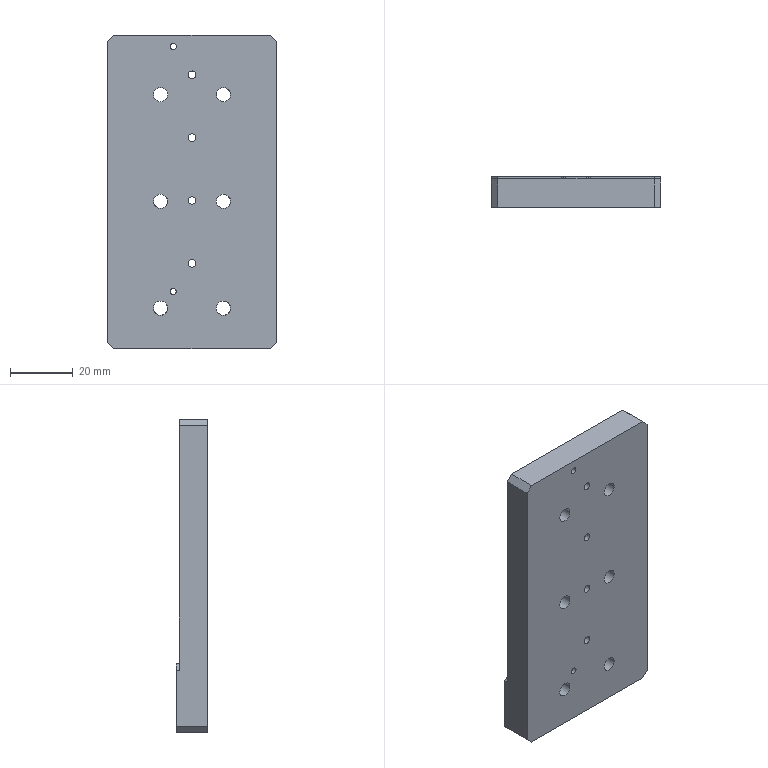Part | 1 solid | 52 faces | box 54 x 10 x 100 mm | volume 47425 mm3 | plane 26 | cylinder 26 | commonest cylinder face diameters 2 x6 4.5 x6 8 x6 2.5 x4 1 x2 3 x2
STEP:
#1=CARTESIAN_POINT('',(137.424,25.392,-106.529));
#2=VERTEX_POINT('',#1);
#3=CARTESIAN_POINT('',(116.923,25.392,-106.529));
#4=VERTEX_POINT('',#3);
#5=CARTESIAN_POINT('',(114.923,25.392,-106.529));
#6=DIRECTION('',(-1.,-0.000000698,0.));
#7=VECTOR('',#6,1000.);
#8=LINE('',#5,#7);
#9=EDGE_CURVE('',#2,#4,#8,.T.);
#10=ORIENTED_EDGE('',*,*,#9,.F.);
#11=CARTESIAN_POINT('',(137.424,26.392,-106.529));
#12=VERTEX_POINT('',#11);
#13=CARTESIAN_POINT('',(137.424,25.892,-106.529));
#14=DIRECTION('',(-0.000000698,1.,0.));
#15=VECTOR('',#14,1000.);
#16=LINE('',#13,#15);
#17=EDGE_CURVE('',#2,#12,#16,.T.);
#18=ORIENTED_EDGE('',*,*,#17,.T.);
#19=CARTESIAN_POINT('',(116.923,26.392,-106.529));
#20=VERTEX_POINT('',#19);
#21=CARTESIAN_POINT('',(114.923,26.392,-106.529));
#22=DIRECTION('',(-1.,-0.000000698,0.));
#23=VECTOR('',#22,1000.);
#24=LINE('',#21,#23);
#25=EDGE_CURVE('',#12,#20,#24,.T.);
#26=ORIENTED_EDGE('',*,*,#25,.T.);
#27=CARTESIAN_POINT('',(116.923,25.392,-106.529));
#28=DIRECTION('',(0.000000698,-1.,0.));
#29=VECTOR('',#28,1000.);
#30=LINE('',#27,#29);
#31=EDGE_CURVE('',#20,#4,#30,.T.);
#32=ORIENTED_EDGE('',*,*,#31,.T.);
#33=EDGE_LOOP('',(#10,#18,#26,#32));
#34=FACE_BOUND('',#33,.T.);
#35=CARTESIAN_POINT('',(114.923,25.392,-106.529));
#36=DIRECTION('',(0.,0.,-1.));
#37=DIRECTION('',(0.,-1.,0.));
#38=AXIS2_PLACEMENT_3D('',#35,#36,#37);
#39=PLANE('',#38);
#40=ADVANCED_FACE('',(#34),#39,.F.);
#41=CARTESIAN_POINT('',(135.923,26.392,-111.729));
#42=VERTEX_POINT('',#41);
#43=CARTESIAN_POINT('',(135.923,26.392,-110.229));
#44=DIRECTION('',(0.000000698,-1.,0.));
#45=DIRECTION('',(-0.000000349,0.,-1.));
#46=AXIS2_PLACEMENT_3D('',#43,#44,#45);
#47=CIRCLE('',#46,1.5);
#48=EDGE_CURVE('',#42,#42,#47,.T.);
#49=ORIENTED_EDGE('',*,*,#48,.T.);
#50=EDGE_LOOP('',(#49));
#51=FACE_BOUND('',#50,.T.);
#52=CARTESIAN_POINT('',(151.923,26.392,-111.529));
#53=VERTEX_POINT('',#52);
#54=CARTESIAN_POINT('',(151.923,26.392,-115.529));
#55=DIRECTION('',(-0.000000698,1.,0.));
#56=DIRECTION('',(0.,0.,1.));
#57=AXIS2_PLACEMENT_3D('',#54,#55,#56);
#58=CIRCLE('',#57,4.);
#59=EDGE_CURVE('',#53,#53,#58,.T.);
#60=ORIENTED_EDGE('',*,*,#59,.F.);
#61=EDGE_LOOP('',(#60));
#62=FACE_BOUND('',#61,.T.);
#63=CARTESIAN_POINT('',(131.923,26.392,-111.529));
#64=VERTEX_POINT('',#63);
#65=CARTESIAN_POINT('',(131.923,26.392,-115.529));
#66=DIRECTION('',(-0.000000698,1.,0.));
#67=DIRECTION('',(0.,0.,1.));
#68=AXIS2_PLACEMENT_3D('',#65,#66,#67);
#69=CIRCLE('',#68,4.);
#70=EDGE_CURVE('',#64,#64,#69,.T.);
#71=ORIENTED_EDGE('',*,*,#70,.F.);
#72=EDGE_LOOP('',(#71));
#73=FACE_BOUND('',#72,.T.);
#74=CARTESIAN_POINT('',(146.051,26.392,-109.062));
#75=VERTEX_POINT('',#74);
#76=CARTESIAN_POINT('',(146.757,26.392,-108.356));
#77=VERTEX_POINT('',#76);
#78=CARTESIAN_POINT('',(146.424,26.392,-108.729));
#79=DIRECTION('',(0.000000698,-1.,0.));
#80=DIRECTION('',(-0.000000349,0.,-1.));
#81=AXIS2_PLACEMENT_3D('',#78,#79,#80);
#82=CIRCLE('',#81,0.5);
#83=EDGE_CURVE('',#75,#77,#82,.T.);
#84=ORIENTED_EDGE('',*,*,#83,.T.);
#85=CARTESIAN_POINT('',(146.424,26.392,-107.611));
#86=VERTEX_POINT('',#85);
#87=CARTESIAN_POINT('',(147.424,26.392,-107.611));
#88=DIRECTION('',(0.000000698,-1.,0.));
#89=DIRECTION('',(1.,0.000000698,0.));
#90=AXIS2_PLACEMENT_3D('',#87,#88,#89);
#91=CIRCLE('',#90,1.);
#92=EDGE_CURVE('',#77,#86,#91,.F.);
#93=ORIENTED_EDGE('',*,*,#92,.T.);
#94=CARTESIAN_POINT('',(146.424,26.392,-106.529));
#95=VERTEX_POINT('',#94);
#96=CARTESIAN_POINT('',(146.424,26.392,-77.529));
#97=DIRECTION('',(0.,0.,-1.));
#98=VECTOR('',#97,1000.);
#99=LINE('',#96,#98);
#100=EDGE_CURVE('',#95,#86,#99,.T.);
#101=ORIENTED_EDGE('',*,*,#100,.F.);
#102=CARTESIAN_POINT('',(166.923,26.392,-106.529));
#103=VERTEX_POINT('',#102);
#104=CARTESIAN_POINT('',(114.923,26.392,-106.529));
#105=DIRECTION('',(-1.,-0.000000698,0.));
#106=VECTOR('',#105,1000.);
#107=LINE('',#104,#106);
#108=EDGE_CURVE('',#103,#95,#107,.T.);
#109=ORIENTED_EDGE('',*,*,#108,.F.);
#110=CARTESIAN_POINT('',(168.923,26.392,-108.529));
#111=VERTEX_POINT('',#110);
#112=CARTESIAN_POINT('',(166.923,26.392,-106.529));
#113=DIRECTION('',(0.7071,0.000000494,-0.7071));
#114=VECTOR('',#113,1000.);
#115=LINE('',#112,#114);
#116=EDGE_CURVE('',#103,#111,#115,.T.);
#117=ORIENTED_EDGE('',*,*,#116,.T.);
#118=CARTESIAN_POINT('',(168.923,26.392,-126.529));
#119=VERTEX_POINT('',#118);
#120=CARTESIAN_POINT('',(168.923,26.392,-128.529));
#121=DIRECTION('',(0.,0.,1.));
#122=VECTOR('',#121,1000.);
#123=LINE('',#120,#122);
#124=EDGE_CURVE('',#119,#111,#123,.T.);
#125=ORIENTED_EDGE('',*,*,#124,.F.);
#126=CARTESIAN_POINT('',(166.923,26.392,-128.529));
#127=VERTEX_POINT('',#126);
#128=CARTESIAN_POINT('',(168.923,26.392,-126.529));
#129=DIRECTION('',(-0.7071,-0.000000494,-0.7071));
#130=VECTOR('',#129,1000.);
#131=LINE('',#128,#130);
#132=EDGE_CURVE('',#119,#127,#131,.T.);
#133=ORIENTED_EDGE('',*,*,#132,.T.);
#134=CARTESIAN_POINT('',(116.923,26.392,-128.529));
#135=VERTEX_POINT('',#134);
#136=CARTESIAN_POINT('',(114.923,26.392,-128.529));
#137=DIRECTION('',(1.,0.000000698,0.));
#138=VECTOR('',#137,1000.);
#139=LINE('',#136,#138);
#140=EDGE_CURVE('',#135,#127,#139,.T.);
#141=ORIENTED_EDGE('',*,*,#140,.F.);
#142=CARTESIAN_POINT('',(114.923,26.392,-126.529));
#143=VERTEX_POINT('',#142);
#144=CARTESIAN_POINT('',(116.923,26.392,-128.529));
#145=DIRECTION('',(-0.7071,-0.000000494,0.7071));
#146=VECTOR('',#145,1000.);
#147=LINE('',#144,#146);
#148=EDGE_CURVE('',#135,#143,#147,.T.);
#149=ORIENTED_EDGE('',*,*,#148,.T.);
#150=CARTESIAN_POINT('',(114.923,26.392,-108.529));
#151=VERTEX_POINT('',#150);
#152=CARTESIAN_POINT('',(114.923,26.392,-128.529));
#153=DIRECTION('',(0.,0.,-1.));
#154=VECTOR('',#153,1000.);
#155=LINE('',#152,#154);
#156=EDGE_CURVE('',#151,#143,#155,.T.);
#157=ORIENTED_EDGE('',*,*,#156,.F.);
#158=CARTESIAN_POINT('',(114.923,26.392,-108.529));
#159=DIRECTION('',(0.7071,0.000000494,0.7071));
#160=VECTOR('',#159,1000.);
#161=LINE('',#158,#160);
#162=EDGE_CURVE('',#151,#20,#161,.T.);
#163=ORIENTED_EDGE('',*,*,#162,.T.);
#164=ORIENTED_EDGE('',*,*,#25,.F.);
#165=CARTESIAN_POINT('',(137.424,26.392,-107.611));
#166=VERTEX_POINT('',#165);
#167=CARTESIAN_POINT('',(137.424,26.392,-77.529));
#168=DIRECTION('',(0.,0.,1.));
#169=VECTOR('',#168,1000.);
#170=LINE('',#167,#169);
#171=EDGE_CURVE('',#166,#12,#170,.T.);
#172=ORIENTED_EDGE('',*,*,#171,.F.);
#173=CARTESIAN_POINT('',(137.091,26.392,-108.357));
#174=VERTEX_POINT('',#173);
#175=CARTESIAN_POINT('',(136.424,26.392,-107.611));
#176=DIRECTION('',(0.000000698,-1.,0.));
#177=DIRECTION('',(1.,0.000000698,0.));
#178=AXIS2_PLACEMENT_3D('',#175,#176,#177);
#179=CIRCLE('',#178,1.);
#180=EDGE_CURVE('',#166,#174,#179,.F.);
#181=ORIENTED_EDGE('',*,*,#180,.T.);
#182=CARTESIAN_POINT('',(137.797,26.392,-109.063));
#183=VERTEX_POINT('',#182);
#184=CARTESIAN_POINT('',(137.424,26.392,-108.729));
#185=DIRECTION('',(0.000000698,-1.,0.));
#186=DIRECTION('',(-0.000000349,0.,-1.));
#187=AXIS2_PLACEMENT_3D('',#184,#185,#186);
#188=CIRCLE('',#187,0.5);
#189=EDGE_CURVE('',#174,#183,#188,.T.);
#190=ORIENTED_EDGE('',*,*,#189,.T.);
#191=CARTESIAN_POINT('',(138.542,26.392,-108.729));
#192=VERTEX_POINT('',#191);
#193=CARTESIAN_POINT('',(138.542,26.392,-109.729));
#194=DIRECTION('',(0.000000698,-1.,0.));
#195=DIRECTION('',(1.,0.000000698,0.));
#196=AXIS2_PLACEMENT_3D('',#193,#194,#195);
#197=CIRCLE('',#196,1.);
#198=EDGE_CURVE('',#183,#192,#197,.F.);
#199=ORIENTED_EDGE('',*,*,#198,.T.);
#200=CARTESIAN_POINT('',(145.306,26.392,-108.729));
#201=VERTEX_POINT('',#200);
#202=CARTESIAN_POINT('',(141.925,26.392,-108.729));
#203=DIRECTION('',(-1.,-0.000000698,0.));
#204=VECTOR('',#203,1000.);
#205=LINE('',#202,#204);
#206=EDGE_CURVE('',#201,#192,#205,.T.);
#207=ORIENTED_EDGE('',*,*,#206,.F.);
#208=CARTESIAN_POINT('',(145.306,26.392,-109.729));
#209=DIRECTION('',(0.000000698,-1.,0.));
#210=DIRECTION('',(1.,0.000000698,0.));
#211=AXIS2_PLACEMENT_3D('',#208,#209,#210);
#212=CIRCLE('',#211,1.);
#213=EDGE_CURVE('',#201,#75,#212,.F.);
#214=ORIENTED_EDGE('',*,*,#213,.T.);
#215=EDGE_LOOP('',(#84,#93,#101,#109,#117,#125,#133,#141,#149,#157,#163,#164,#172,#181,#190,#199,#207,#214));
#216=FACE_BOUND('',#215,.T.);
#217=CARTESIAN_POINT('',(141.923,26.392,-77.529));
#218=DIRECTION('',(0.000000698,-1.,0.));
#219=DIRECTION('',(0.,0.,-1.));
#220=AXIS2_PLACEMENT_3D('',#217,#218,#219);
#221=PLANE('',#220);
#222=ADVANCED_FACE('',(#51,#62,#73,#216),#221,.F.);
#223=CARTESIAN_POINT('',(166.923,16.392,-28.529));
#224=VERTEX_POINT('',#223);
#225=CARTESIAN_POINT('',(116.923,16.392,-28.529));
#226=VERTEX_POINT('',#225);
#227=CARTESIAN_POINT('',(114.923,16.392,-28.529));
#228=DIRECTION('',(-1.,-0.000000698,0.));
#229=VECTOR('',#228,1000.);
#230=LINE('',#227,#229);
#231=EDGE_CURVE('',#224,#226,#230,.T.);
#232=ORIENTED_EDGE('',*,*,#231,.F.);
#233=CARTESIAN_POINT('',(166.923,25.392,-28.529));
#234=VERTEX_POINT('',#233);
#235=CARTESIAN_POINT('',(166.923,16.392,-28.529));
#236=DIRECTION('',(-0.000000698,1.,0.));
#237=VECTOR('',#236,1000.);
#238=LINE('',#235,#237);
#239=EDGE_CURVE('',#224,#234,#238,.T.);
#240=ORIENTED_EDGE('',*,*,#239,.T.);
#241=CARTESIAN_POINT('',(116.923,25.392,-28.529));
#242=VERTEX_POINT('',#241);
#243=CARTESIAN_POINT('',(114.923,25.392,-28.529));
#244=DIRECTION('',(1.,0.000000698,0.));
#245=VECTOR('',#244,1000.);
#246=LINE('',#243,#245);
#247=EDGE_CURVE('',#242,#234,#246,.T.);
#248=ORIENTED_EDGE('',*,*,#247,.F.);
#249=CARTESIAN_POINT('',(116.923,16.392,-28.529));
#250=DIRECTION('',(0.000000698,-1.,0.));
#251=VECTOR('',#250,1000.);
#252=LINE('',#249,#251);
#253=EDGE_CURVE('',#242,#226,#252,.T.);
#254=ORIENTED_EDGE('',*,*,#253,.T.);
#255=EDGE_LOOP('',(#232,#240,#248,#254));
#256=FACE_BOUND('',#255,.T.);
#257=CARTESIAN_POINT('',(114.923,16.392,-28.529));
#258=DIRECTION('',(0.,0.,-1.));
#259=DIRECTION('',(0.,-1.,0.));
#260=AXIS2_PLACEMENT_3D('',#257,#258,#259);
#261=PLANE('',#260);
#262=ADVANCED_FACE('',(#256),#261,.F.);
#263=CARTESIAN_POINT('',(114.923,16.392,-30.529));
#264=VERTEX_POINT('',#263);
#265=CARTESIAN_POINT('',(114.923,16.392,-126.529));
#266=VERTEX_POINT('',#265);
#267=CARTESIAN_POINT('',(114.923,16.392,-128.529));
#268=DIRECTION('',(0.,0.,-1.));
#269=VECTOR('',#268,1000.);
#270=LINE('',#267,#269);
#271=EDGE_CURVE('',#264,#266,#270,.T.);
#272=ORIENTED_EDGE('',*,*,#271,.F.);
#273=CARTESIAN_POINT('',(114.923,25.392,-30.529));
#274=VERTEX_POINT('',#273);
#275=CARTESIAN_POINT('',(114.923,16.392,-30.529));
#276=DIRECTION('',(-0.000000698,1.,0.));
#277=VECTOR('',#276,1000.);
#278=LINE('',#275,#277);
#279=EDGE_CURVE('',#264,#274,#278,.T.);
#280=ORIENTED_EDGE('',*,*,#279,.T.);
#281=CARTESIAN_POINT('',(114.923,25.392,-108.529));
#282=VERTEX_POINT('',#281);
#283=CARTESIAN_POINT('',(114.923,25.392,-26.529));
#284=DIRECTION('',(0.,0.,1.));
#285=VECTOR('',#284,1000.);
#286=LINE('',#283,#285);
#287=EDGE_CURVE('',#282,#274,#286,.T.);
#288=ORIENTED_EDGE('',*,*,#287,.F.);
#289=CARTESIAN_POINT('',(114.923,16.392,-108.529));
#290=DIRECTION('',(-0.000000698,1.,0.));
#291=VECTOR('',#290,1000.);
#292=LINE('',#289,#291);
#293=EDGE_CURVE('',#282,#151,#292,.T.);
#294=ORIENTED_EDGE('',*,*,#293,.T.);
#295=ORIENTED_EDGE('',*,*,#156,.T.);
#296=CARTESIAN_POINT('',(114.923,16.392,-126.529));
#297=DIRECTION('',(0.000000698,-1.,0.));
#298=VECTOR('',#297,1000.);
#299=LINE('',#296,#298);
#300=EDGE_CURVE('',#143,#266,#299,.T.);
#301=ORIENTED_EDGE('',*,*,#300,.T.);
#302=EDGE_LOOP('',(#272,#280,#288,#294,#295,#301));
#303=FACE_BOUND('',#302,.T.);
#304=CARTESIAN_POINT('',(114.923,16.392,-128.529));
#305=DIRECTION('',(1.,0.000000698,0.));
#306=DIRECTION('',(0.,0.000000533,-1.));
#307=AXIS2_PLACEMENT_3D('',#304,#305,#306);
#308=PLANE('',#307);
#309=ADVANCED_FACE('',(#303),#308,.F.);
#310=ORIENTED_EDGE('',*,*,#140,.T.);
#311=CARTESIAN_POINT('',(166.923,16.392,-128.529));
#312=VERTEX_POINT('',#311);
#313=CARTESIAN_POINT('',(166.923,16.392,-128.529));
#314=DIRECTION('',(0.000000698,-1.,0.));
#315=VECTOR('',#314,1000.);
#316=LINE('',#313,#315);
#317=EDGE_CURVE('',#127,#312,#316,.T.);
#318=ORIENTED_EDGE('',*,*,#317,.T.);
#319=CARTESIAN_POINT('',(116.923,16.392,-128.529));
#320=VERTEX_POINT('',#319);
#321=CARTESIAN_POINT('',(114.923,16.392,-128.529));
#322=DIRECTION('',(1.,0.000000698,0.));
#323=VECTOR('',#322,1000.);
#324=LINE('',#321,#323);
#325=EDGE_CURVE('',#320,#312,#324,.T.);
#326=ORIENTED_EDGE('',*,*,#325,.F.);
#327=CARTESIAN_POINT('',(116.923,16.392,-128.529));
#328=DIRECTION('',(-0.000000698,1.,0.));
#329=VECTOR('',#328,1000.);
#330=LINE('',#327,#329);
#331=EDGE_CURVE('',#320,#135,#330,.T.);
#332=ORIENTED_EDGE('',*,*,#331,.T.);
#333=EDGE_LOOP('',(#310,#318,#326,#332));
#334=FACE_BOUND('',#333,.T.);
#335=CARTESIAN_POINT('',(114.923,16.392,-128.529));
#336=DIRECTION('',(0.,0.,1.));
#337=DIRECTION('',(1.,0.,0.));
#338=AXIS2_PLACEMENT_3D('',#335,#336,#337);
#339=PLANE('',#338);
#340=ADVANCED_FACE('',(#334),#339,.F.);
#341=CARTESIAN_POINT('',(168.923,25.392,-30.529));
#342=VERTEX_POINT('',#341);
#343=CARTESIAN_POINT('',(168.923,25.392,-108.529));
#344=VERTEX_POINT('',#343);
#345=CARTESIAN_POINT('',(168.923,25.392,-26.529));
#346=DIRECTION('',(0.,0.,-1.));
#347=VECTOR('',#346,1000.);
#348=LINE('',#345,#347);
#349=EDGE_CURVE('',#342,#344,#348,.T.);
#350=ORIENTED_EDGE('',*,*,#349,.F.);
#351=CARTESIAN_POINT('',(168.923,16.392,-30.529));
#352=VERTEX_POINT('',#351);
#353=CARTESIAN_POINT('',(168.923,16.392,-30.529));
#354=DIRECTION('',(0.000000698,-1.,0.));
#355=VECTOR('',#354,1000.);
#356=LINE('',#353,#355);
#357=EDGE_CURVE('',#342,#352,#356,.T.);
#358=ORIENTED_EDGE('',*,*,#357,.T.);
#359=CARTESIAN_POINT('',(168.923,16.392,-126.529));
#360=VERTEX_POINT('',#359);
#361=CARTESIAN_POINT('',(168.923,16.392,-128.529));
#362=DIRECTION('',(0.,0.,1.));
#363=VECTOR('',#362,1000.);
#364=LINE('',#361,#363);
#365=EDGE_CURVE('',#360,#352,#364,.T.);
#366=ORIENTED_EDGE('',*,*,#365,.F.);
#367=CARTESIAN_POINT('',(168.923,16.392,-126.529));
#368=DIRECTION('',(-0.000000698,1.,0.));
#369=VECTOR('',#368,1000.);
#370=LINE('',#367,#369);
#371=EDGE_CURVE('',#360,#119,#370,.T.);
#372=ORIENTED_EDGE('',*,*,#371,.T.);
#373=ORIENTED_EDGE('',*,*,#124,.T.);
#374=CARTESIAN_POINT('',(168.923,16.392,-108.529));
#375=DIRECTION('',(0.000000698,-1.,0.));
#376=VECTOR('',#375,1000.);
#377=LINE('',#374,#376);
#378=EDGE_CURVE('',#111,#344,#377,.T.);
#379=ORIENTED_EDGE('',*,*,#378,.T.);
#380=EDGE_LOOP('',(#350,#358,#366,#372,#373,#379));
#381=FACE_BOUND('',#380,.T.);
#382=CARTESIAN_POINT('',(168.923,16.392,-128.529));
#383=DIRECTION('',(-1.,-0.000000698,0.));
#384=DIRECTION('',(-0.000000698,1.,0.));
#385=AXIS2_PLACEMENT_3D('',#382,#383,#384);
#386=PLANE('',#385);
#387=ADVANCED_FACE('',(#381),#386,.F.);
#388=CARTESIAN_POINT('',(135.923,16.392,-33.229));
#389=VERTEX_POINT('',#388);
#390=CARTESIAN_POINT('',(135.923,16.392,-32.229));
#391=DIRECTION('',(-0.000000698,1.,0.));
#392=DIRECTION('',(-0.000000349,0.,-1.));
#393=AXIS2_PLACEMENT_3D('',#390,#391,#392);
#394=CIRCLE('',#393,1.);
#395=EDGE_CURVE('',#389,#389,#394,.T.);
#396=ORIENTED_EDGE('',*,*,#395,.T.);
#397=EDGE_LOOP('',(#396));
#398=FACE_BOUND('',#397,.T.);
#399=CARTESIAN_POINT('',(135.923,16.392,-111.229));
#400=VERTEX_POINT('',#399);
#401=CARTESIAN_POINT('',(135.923,16.392,-110.229));
#402=DIRECTION('',(-0.000000698,1.,0.));
#403=DIRECTION('',(-0.000000349,0.,-1.));
#404=AXIS2_PLACEMENT_3D('',#401,#402,#403);
#405=CIRCLE('',#404,1.);
#406=EDGE_CURVE('',#400,#400,#405,.T.);
#407=ORIENTED_EDGE('',*,*,#406,.T.);
#408=EDGE_LOOP('',(#407));
#409=FACE_BOUND('',#408,.T.);
#410=CARTESIAN_POINT('',(141.923,16.392,-62.479));
#411=VERTEX_POINT('',#410);
#412=CARTESIAN_POINT('',(141.923,16.392,-61.229));
#413=DIRECTION('',(-0.000000698,1.,0.));
#414=DIRECTION('',(-0.000000349,0.,-1.));
#415=AXIS2_PLACEMENT_3D('',#412,#413,#414);
#416=CIRCLE('',#415,1.25);
#417=EDGE_CURVE('',#411,#411,#416,.T.);
#418=ORIENTED_EDGE('',*,*,#417,.T.);
#419=EDGE_LOOP('',(#418));
#420=FACE_BOUND('',#419,.T.);
#421=CARTESIAN_POINT('',(141.923,16.392,-42.479));
#422=VERTEX_POINT('',#421);
#423=CARTESIAN_POINT('',(141.923,16.392,-41.229));
#424=DIRECTION('',(-0.000000698,1.,0.));
#425=DIRECTION('',(-0.000000349,0.,-1.));
#426=AXIS2_PLACEMENT_3D('',#423,#424,#425);
#427=CIRCLE('',#426,1.25);
#428=EDGE_CURVE('',#422,#422,#427,.T.);
#429=ORIENTED_EDGE('',*,*,#428,.T.);
#430=EDGE_LOOP('',(#429));
#431=FACE_BOUND('',#430,.T.);
#432=CARTESIAN_POINT('',(141.923,16.392,-82.479));
#433=VERTEX_POINT('',#432);
#434=CARTESIAN_POINT('',(141.923,16.392,-81.229));
#435=DIRECTION('',(-0.000000698,1.,0.));
#436=DIRECTION('',(-0.000000349,0.,-1.));
#437=AXIS2_PLACEMENT_3D('',#434,#435,#436);
#438=CIRCLE('',#437,1.25);
#439=EDGE_CURVE('',#433,#433,#438,.T.);
#440=ORIENTED_EDGE('',*,*,#439,.T.);
#441=EDGE_LOOP('',(#440));
#442=FACE_BOUND('',#441,.T.);
#443=CARTESIAN_POINT('',(141.923,16.392,-102.479));
#444=VERTEX_POINT('',#443);
#445=CARTESIAN_POINT('',(141.923,16.392,-101.229));
#446=DIRECTION('',(-0.000000698,1.,0.));
#447=DIRECTION('',(-0.000000349,0.,-1.));
#448=AXIS2_PLACEMENT_3D('',#445,#446,#447);
#449=CIRCLE('',#448,1.25);
#450=EDGE_CURVE('',#444,#444,#449,.T.);
#451=ORIENTED_EDGE('',*,*,#450,.T.);
#452=EDGE_LOOP('',(#451));
#453=FACE_BOUND('',#452,.T.);
#454=CARTESIAN_POINT('',(131.923,16.392,-45.279));
#455=VERTEX_POINT('',#454);
#456=CARTESIAN_POINT('',(131.923,16.392,-47.529));
#457=DIRECTION('',(-0.000000698,1.,0.));
#458=DIRECTION('',(0.,0.,1.));
#459=AXIS2_PLACEMENT_3D('',#456,#457,#458);
#460=CIRCLE('',#459,2.25);
#461=EDGE_CURVE('',#455,#455,#460,.T.);
#462=ORIENTED_EDGE('',*,*,#461,.T.);
#463=EDGE_LOOP('',(#462));
#464=FACE_BOUND('',#463,.T.);
#465=CARTESIAN_POINT('',(151.923,16.392,-45.279));
#466=VERTEX_POINT('',#465);
#467=CARTESIAN_POINT('',(151.923,16.392,-47.529));
#468=DIRECTION('',(-0.000000698,1.,0.));
#469=DIRECTION('',(0.,0.,1.));
#470=AXIS2_PLACEMENT_3D('',#467,#468,#469);
#471=CIRCLE('',#470,2.25);
#472=EDGE_CURVE('',#466,#466,#471,.T.);
#473=ORIENTED_EDGE('',*,*,#472,.T.);
#474=EDGE_LOOP('',(#473));
#475=FACE_BOUND('',#474,.T.);
#476=CARTESIAN_POINT('',(131.923,16.392,-79.279));
#477=VERTEX_POINT('',#476);
#478=CARTESIAN_POINT('',(131.923,16.392,-81.529));
#479=DIRECTION('',(-0.000000698,1.,0.));
#480=DIRECTION('',(0.,0.,1.));
#481=AXIS2_PLACEMENT_3D('',#478,#479,#480);
#482=CIRCLE('',#481,2.25);
#483=EDGE_CURVE('',#477,#477,#482,.T.);
#484=ORIENTED_EDGE('',*,*,#483,.T.);
#485=EDGE_LOOP('',(#484));
#486=FACE_BOUND('',#485,.T.);
#487=CARTESIAN_POINT('',(151.923,16.392,-79.279));
#488=VERTEX_POINT('',#487);
#489=CARTESIAN_POINT('',(151.923,16.392,-81.529));
#490=DIRECTION('',(-0.000000698,1.,0.));
#491=DIRECTION('',(0.,0.,1.));
#492=AXIS2_PLACEMENT_3D('',#489,#490,#491);
#493=CIRCLE('',#492,2.25);
#494=EDGE_CURVE('',#488,#488,#493,.T.);
#495=ORIENTED_EDGE('',*,*,#494,.T.);
#496=EDGE_LOOP('',(#495));
#497=FACE_BOUND('',#496,.T.);
#498=CARTESIAN_POINT('',(131.923,16.392,-113.279));
#499=VERTEX_POINT('',#498);
#500=CARTESIAN_POINT('',(131.923,16.392,-115.529));
#501=DIRECTION('',(-0.000000698,1.,0.));
#502=DIRECTION('',(0.,0.,1.));
#503=AXIS2_PLACEMENT_3D('',#500,#501,#502);
#504=CIRCLE('',#503,2.25);
#505=EDGE_CURVE('',#499,#499,#504,.T.);
#506=ORIENTED_EDGE('',*,*,#505,.T.);
#507=EDGE_LOOP('',(#506));
#508=FACE_BOUND('',#507,.T.);
#509=CARTESIAN_POINT('',(151.923,16.392,-113.279));
#510=VERTEX_POINT('',#509);
#511=CARTESIAN_POINT('',(151.923,16.392,-115.529));
#512=DIRECTION('',(-0.000000698,1.,0.));
#513=DIRECTION('',(0.,0.,1.));
#514=AXIS2_PLACEMENT_3D('',#511,#512,#513);
#515=CIRCLE('',#514,2.25);
#516=EDGE_CURVE('',#510,#510,#515,.T.);
#517=ORIENTED_EDGE('',*,*,#516,.T.);
#518=EDGE_LOOP('',(#517));
#519=FACE_BOUND('',#518,.T.);
#520=ORIENTED_EDGE('',*,*,#365,.T.);
#521=CARTESIAN_POINT('',(178.923,16.392,-40.529));
#522=DIRECTION('',(-0.7071,-0.000000494,0.7071));
#523=VECTOR('',#522,1000.);
#524=LINE('',#521,#523);
#525=EDGE_CURVE('',#352,#224,#524,.T.);
#526=ORIENTED_EDGE('',*,*,#525,.T.);
#527=ORIENTED_EDGE('',*,*,#231,.T.);
#528=CARTESIAN_POINT('',(104.923,16.392,-40.529));
#529=DIRECTION('',(-0.7071,-0.000000494,-0.7071));
#530=VECTOR('',#529,1000.);
#531=LINE('',#528,#530);
#532=EDGE_CURVE('',#226,#264,#531,.T.);
#533=ORIENTED_EDGE('',*,*,#532,.T.);
#534=ORIENTED_EDGE('',*,*,#271,.T.);
#535=CARTESIAN_POINT('',(103.923,16.392,-115.529));
#536=DIRECTION('',(0.7071,0.000000494,-0.7071));
#537=VECTOR('',#536,1000.);
#538=LINE('',#535,#537);
#539=EDGE_CURVE('',#266,#320,#538,.T.);
#540=ORIENTED_EDGE('',*,*,#539,.T.);
#541=ORIENTED_EDGE('',*,*,#325,.T.);
#542=CARTESIAN_POINT('',(179.923,16.392,-115.529));
#543=DIRECTION('',(0.7071,0.000000494,0.7071));
#544=VECTOR('',#543,1000.);
#545=LINE('',#542,#544);
#546=EDGE_CURVE('',#312,#360,#545,.T.);
#547=ORIENTED_EDGE('',*,*,#546,.T.);
#548=EDGE_LOOP('',(#520,#526,#527,#533,#534,#540,#541,#547));
#549=FACE_BOUND('',#548,.T.);
#550=CARTESIAN_POINT('',(141.923,16.392,-77.529));
#551=DIRECTION('',(0.000000698,-1.,0.));
#552=DIRECTION('',(0.,0.,-1.));
#553=AXIS2_PLACEMENT_3D('',#550,#551,#552);
#554=PLANE('',#553);
#555=ADVANCED_FACE('',(#398,#409,#420,#431,#442,#453,#464,#475,#486,#497,#508,#519,#549),#554,.T.);
#556=CARTESIAN_POINT('',(154.173,20.392,-115.529));
#557=VERTEX_POINT('',#556);
#558=CARTESIAN_POINT('',(151.923,20.392,-115.529));
#559=DIRECTION('',(-0.000000698,1.,0.));
#560=DIRECTION('',(1.,0.000000698,0.));
#561=AXIS2_PLACEMENT_3D('',#558,#559,#560);
#562=CIRCLE('',#561,2.25);
#563=EDGE_CURVE('',#557,#557,#562,.T.);
#564=ORIENTED_EDGE('',*,*,#563,.F.);
#565=EDGE_LOOP('',(#564));
#566=FACE_BOUND('',#565,.T.);
#567=CARTESIAN_POINT('',(155.923,20.392,-115.529));
#568=VERTEX_POINT('',#567);
#569=CARTESIAN_POINT('',(151.923,20.392,-115.529));
#570=DIRECTION('',(-0.000000698,1.,0.));
#571=DIRECTION('',(1.,0.000000698,0.));
#572=AXIS2_PLACEMENT_3D('',#569,#570,#571);
#573=CIRCLE('',#572,4.);
#574=EDGE_CURVE('',#568,#568,#573,.T.);
#575=ORIENTED_EDGE('',*,*,#574,.T.);
#576=EDGE_LOOP('',(#575));
#577=FACE_BOUND('',#576,.T.);
#578=CARTESIAN_POINT('',(131.923,20.392,-49.779));
#579=DIRECTION('',(0.000000698,-1.,0.));
#580=DIRECTION('',(0.,0.,-1.));
#581=AXIS2_PLACEMENT_3D('',#578,#579,#580);
#582=PLANE('',#581);
#583=ADVANCED_FACE('',(#566,#577),#582,.F.);
#584=CARTESIAN_POINT('',(134.173,20.392,-115.529));
#585=VERTEX_POINT('',#584);
#586=CARTESIAN_POINT('',(131.923,20.392,-115.529));
#587=DIRECTION('',(-0.000000698,1.,0.));
#588=DIRECTION('',(1.,0.000000698,0.));
#589=AXIS2_PLACEMENT_3D('',#586,#587,#588);
#590=CIRCLE('',#589,2.25);
#591=EDGE_CURVE('',#585,#585,#590,.T.);
#592=ORIENTED_EDGE('',*,*,#591,.F.);
#593=EDGE_LOOP('',(#592));
#594=FACE_BOUND('',#593,.T.);
#595=CARTESIAN_POINT('',(135.923,20.392,-115.529));
#596=VERTEX_POINT('',#595);
#597=CARTESIAN_POINT('',(131.923,20.392,-115.529));
#598=DIRECTION('',(-0.000000698,1.,0.));
#599=DIRECTION('',(1.,0.000000698,0.));
#600=AXIS2_PLACEMENT_3D('',#597,#598,#599);
#601=CIRCLE('',#600,4.);
#602=EDGE_CURVE('',#596,#596,#601,.T.);
#603=ORIENTED_EDGE('',*,*,#602,.T.);
#604=EDGE_LOOP('',(#603));
#605=FACE_BOUND('',#604,.T.);
#606=CARTESIAN_POINT('',(131.923,20.392,-49.779));
#607=DIRECTION('',(0.000000698,-1.,0.));
#608=DIRECTION('',(0.,0.,-1.));
#609=AXIS2_PLACEMENT_3D('',#606,#607,#608);
#610=PLANE('',#609);
#611=ADVANCED_FACE('',(#594,#605),#610,.F.);
#612=CARTESIAN_POINT('',(154.173,20.392,-81.529));
#613=VERTEX_POINT('',#612);
#614=CARTESIAN_POINT('',(151.923,20.392,-81.529));
#615=DIRECTION('',(-0.000000698,1.,0.));
#616=DIRECTION('',(1.,0.000000698,0.));
#617=AXIS2_PLACEMENT_3D('',#614,#615,#616);
#618=CIRCLE('',#617,2.25);
#619=EDGE_CURVE('',#613,#613,#618,.T.);
#620=ORIENTED_EDGE('',*,*,#619,.F.);
#621=EDGE_LOOP('',(#620));
#622=FACE_BOUND('',#621,.T.);
#623=CARTESIAN_POINT('',(155.923,20.392,-81.529));
#624=VERTEX_POINT('',#623);
#625=CARTESIAN_POINT('',(151.923,20.392,-81.529));
#626=DIRECTION('',(-0.000000698,1.,0.));
#627=DIRECTION('',(1.,0.000000698,0.));
#628=AXIS2_PLACEMENT_3D('',#625,#626,#627);
#629=CIRCLE('',#628,4.);
#630=EDGE_CURVE('',#624,#624,#629,.T.);
#631=ORIENTED_EDGE('',*,*,#630,.T.);
#632=EDGE_LOOP('',(#631));
#633=FACE_BOUND('',#632,.T.);
#634=CARTESIAN_POINT('',(131.923,20.392,-49.779));
#635=DIRECTION('',(0.000000698,-1.,0.));
#636=DIRECTION('',(0.,0.,-1.));
#637=AXIS2_PLACEMENT_3D('',#634,#635,#636);
#638=PLANE('',#637);
#639=ADVANCED_FACE('',(#622,#633),#638,.F.);
#640=CARTESIAN_POINT('',(134.173,20.392,-81.529));
#641=VERTEX_POINT('',#640);
#642=CARTESIAN_POINT('',(131.923,20.392,-81.529));
#643=DIRECTION('',(-0.000000698,1.,0.));
#644=DIRECTION('',(1.,0.000000698,0.));
#645=AXIS2_PLACEMENT_3D('',#642,#643,#644);
#646=CIRCLE('',#645,2.25);
#647=EDGE_CURVE('',#641,#641,#646,.T.);
#648=ORIENTED_EDGE('',*,*,#647,.F.);
#649=EDGE_LOOP('',(#648));
#650=FACE_BOUND('',#649,.T.);
#651=CARTESIAN_POINT('',(135.923,20.392,-81.529));
#652=VERTEX_POINT('',#651);
#653=CARTESIAN_POINT('',(131.923,20.392,-81.529));
#654=DIRECTION('',(-0.000000698,1.,0.));
#655=DIRECTION('',(1.,0.000000698,0.));
#656=AXIS2_PLACEMENT_3D('',#653,#654,#655);
#657=CIRCLE('',#656,4.);
#658=EDGE_CURVE('',#652,#652,#657,.T.);
#659=ORIENTED_EDGE('',*,*,#658,.T.);
#660=EDGE_LOOP('',(#659));
#661=FACE_BOUND('',#660,.T.);
#662=CARTESIAN_POINT('',(131.923,20.392,-49.779));
#663=DIRECTION('',(0.000000698,-1.,0.));
#664=DIRECTION('',(0.,0.,-1.));
#665=AXIS2_PLACEMENT_3D('',#662,#663,#664);
#666=PLANE('',#665);
#667=ADVANCED_FACE('',(#650,#661),#666,.F.);
#668=CARTESIAN_POINT('',(154.173,20.392,-47.529));
#669=VERTEX_POINT('',#668);
#670=CARTESIAN_POINT('',(151.923,20.392,-47.529));
#671=DIRECTION('',(-0.000000698,1.,0.));
#672=DIRECTION('',(1.,0.000000698,0.));
#673=AXIS2_PLACEMENT_3D('',#670,#671,#672);
#674=CIRCLE('',#673,2.25);
#675=EDGE_CURVE('',#669,#669,#674,.T.);
#676=ORIENTED_EDGE('',*,*,#675,.F.);
#677=EDGE_LOOP('',(#676));
#678=FACE_BOUND('',#677,.T.);
#679=CARTESIAN_POINT('',(155.923,20.392,-47.529));
#680=VERTEX_POINT('',#679);
#681=CARTESIAN_POINT('',(151.923,20.392,-47.529));
#682=DIRECTION('',(-0.000000698,1.,0.));
#683=DIRECTION('',(1.,0.000000698,0.));
#684=AXIS2_PLACEMENT_3D('',#681,#682,#683);
#685=CIRCLE('',#684,4.);
#686=EDGE_CURVE('',#680,#680,#685,.T.);
#687=ORIENTED_EDGE('',*,*,#686,.T.);
#688=EDGE_LOOP('',(#687));
#689=FACE_BOUND('',#688,.T.);
#690=CARTESIAN_POINT('',(131.923,20.392,-49.779));
#691=DIRECTION('',(0.000000698,-1.,0.));
#692=DIRECTION('',(0.,0.,-1.));
#693=AXIS2_PLACEMENT_3D('',#690,#691,#692);
#694=PLANE('',#693);
#695=ADVANCED_FACE('',(#678,#689),#694,.F.);
#696=CARTESIAN_POINT('',(131.923,20.392,-45.279));
#697=VERTEX_POINT('',#696);
#698=CARTESIAN_POINT('',(131.923,20.392,-47.529));
#699=DIRECTION('',(-0.000000698,1.,0.));
#700=DIRECTION('',(0.,0.,1.));
#701=AXIS2_PLACEMENT_3D('',#698,#699,#700);
#702=CIRCLE('',#701,2.25);
#703=EDGE_CURVE('',#697,#697,#702,.T.);
#704=ORIENTED_EDGE('',*,*,#703,.F.);
#705=EDGE_LOOP('',(#704));
#706=FACE_BOUND('',#705,.T.);
#707=CARTESIAN_POINT('',(131.923,20.392,-43.529));
#708=VERTEX_POINT('',#707);
#709=CARTESIAN_POINT('',(131.923,20.392,-47.529));
#710=DIRECTION('',(-0.000000698,1.,0.));
#711=DIRECTION('',(0.,0.,1.));
#712=AXIS2_PLACEMENT_3D('',#709,#710,#711);
#713=CIRCLE('',#712,4.);
#714=EDGE_CURVE('',#708,#708,#713,.T.);
#715=ORIENTED_EDGE('',*,*,#714,.T.);
#716=EDGE_LOOP('',(#715));
#717=FACE_BOUND('',#716,.T.);
#718=CARTESIAN_POINT('',(131.923,20.392,-49.779));
#719=DIRECTION('',(0.000000698,-1.,0.));
#720=DIRECTION('',(0.,0.,-1.));
#721=AXIS2_PLACEMENT_3D('',#718,#719,#720);
#722=PLANE('',#721);
#723=ADVANCED_FACE('',(#706,#717),#722,.F.);
#724=ORIENTED_EDGE('',*,*,#247,.T.);
#725=CARTESIAN_POINT('',(178.923,25.392,-40.529));
#726=DIRECTION('',(0.7071,0.000000494,-0.7071));
#727=VECTOR('',#726,1000.);
#728=LINE('',#725,#727);
#729=EDGE_CURVE('',#234,#342,#728,.T.);
#730=ORIENTED_EDGE('',*,*,#729,.T.);
#731=ORIENTED_EDGE('',*,*,#349,.T.);
#732=CARTESIAN_POINT('',(166.923,25.392,-106.529));
#733=VERTEX_POINT('',#732);
#734=CARTESIAN_POINT('',(166.923,25.392,-106.529));
#735=DIRECTION('',(-0.7071,-0.000000494,0.7071));
#736=VECTOR('',#735,1000.);
#737=LINE('',#734,#736);
#738=EDGE_CURVE('',#344,#733,#737,.T.);
#739=ORIENTED_EDGE('',*,*,#738,.T.);
#740=CARTESIAN_POINT('',(146.424,25.392,-106.529));
#741=VERTEX_POINT('',#740);
#742=CARTESIAN_POINT('',(114.923,25.392,-106.529));
#743=DIRECTION('',(-1.,-0.000000698,0.));
#744=VECTOR('',#743,1000.);
#745=LINE('',#742,#744);
#746=EDGE_CURVE('',#733,#741,#745,.T.);
#747=ORIENTED_EDGE('',*,*,#746,.T.);
#748=CARTESIAN_POINT('',(146.424,25.392,-107.611));
#749=VERTEX_POINT('',#748);
#750=CARTESIAN_POINT('',(146.424,25.392,-77.529));
#751=DIRECTION('',(0.,0.,1.));
#752=VECTOR('',#751,1000.);
#753=LINE('',#750,#752);
#754=EDGE_CURVE('',#749,#741,#753,.T.);
#755=ORIENTED_EDGE('',*,*,#754,.F.);
#756=CARTESIAN_POINT('',(146.757,25.392,-108.356));
#757=VERTEX_POINT('',#756);
#758=CARTESIAN_POINT('',(147.424,25.392,-107.611));
#759=DIRECTION('',(-0.000000698,1.,0.));
#760=DIRECTION('',(-1.,-0.000000698,0.));
#761=AXIS2_PLACEMENT_3D('',#758,#759,#760);
#762=CIRCLE('',#761,1.);
#763=EDGE_CURVE('',#749,#757,#762,.F.);
#764=ORIENTED_EDGE('',*,*,#763,.T.);
#765=CARTESIAN_POINT('',(146.051,25.392,-109.062));
#766=VERTEX_POINT('',#765);
#767=CARTESIAN_POINT('',(146.424,25.392,-108.729));
#768=DIRECTION('',(-0.000000698,1.,0.));
#769=DIRECTION('',(1.,0.000000698,-0.000000698));
#770=AXIS2_PLACEMENT_3D('',#767,#768,#769);
#771=CIRCLE('',#770,0.5);
#772=EDGE_CURVE('',#757,#766,#771,.T.);
#773=ORIENTED_EDGE('',*,*,#772,.T.);
#774=CARTESIAN_POINT('',(145.306,25.392,-108.729));
#775=VERTEX_POINT('',#774);
#776=CARTESIAN_POINT('',(145.306,25.392,-109.729));
#777=DIRECTION('',(-0.000000698,1.,0.));
#778=DIRECTION('',(-1.,-0.000000698,0.));
#779=AXIS2_PLACEMENT_3D('',#776,#777,#778);
#780=CIRCLE('',#779,1.);
#781=EDGE_CURVE('',#766,#775,#780,.F.);
#782=ORIENTED_EDGE('',*,*,#781,.T.);
#783=CARTESIAN_POINT('',(138.542,25.392,-108.729));
#784=VERTEX_POINT('',#783);
#785=CARTESIAN_POINT('',(141.925,25.392,-108.729));
#786=DIRECTION('',(1.,0.000000698,0.));
#787=VECTOR('',#786,1000.);
#788=LINE('',#785,#787);
#789=EDGE_CURVE('',#784,#775,#788,.T.);
#790=ORIENTED_EDGE('',*,*,#789,.F.);
#791=CARTESIAN_POINT('',(137.797,25.392,-109.063));
#792=VERTEX_POINT('',#791);
#793=CARTESIAN_POINT('',(138.542,25.392,-109.729));
#794=DIRECTION('',(-0.000000698,1.,0.));
#795=DIRECTION('',(-1.,-0.000000698,0.));
#796=AXIS2_PLACEMENT_3D('',#793,#794,#795);
#797=CIRCLE('',#796,1.);
#798=EDGE_CURVE('',#784,#792,#797,.F.);
#799=ORIENTED_EDGE('',*,*,#798,.T.);
#800=CARTESIAN_POINT('',(137.091,25.392,-108.357));
#801=VERTEX_POINT('',#800);
#802=CARTESIAN_POINT('',(137.424,25.392,-108.729));
#803=DIRECTION('',(-0.000000698,1.,0.));
#804=DIRECTION('',(1.,0.000000698,-0.000000698));
#805=AXIS2_PLACEMENT_3D('',#802,#803,#804);
#806=CIRCLE('',#805,0.5);
#807=EDGE_CURVE('',#792,#801,#806,.T.);
#808=ORIENTED_EDGE('',*,*,#807,.T.);
#809=CARTESIAN_POINT('',(137.424,25.392,-107.611));
#810=VERTEX_POINT('',#809);
#811=CARTESIAN_POINT('',(136.424,25.392,-107.611));
#812=DIRECTION('',(-0.000000698,1.,0.));
#813=DIRECTION('',(-1.,-0.000000698,0.));
#814=AXIS2_PLACEMENT_3D('',#811,#812,#813);
#815=CIRCLE('',#814,1.);
#816=EDGE_CURVE('',#801,#810,#815,.F.);
#817=ORIENTED_EDGE('',*,*,#816,.T.);
#818=CARTESIAN_POINT('',(137.424,25.392,-77.529));
#819=DIRECTION('',(0.,0.,-1.));
#820=VECTOR('',#819,1000.);
#821=LINE('',#818,#820);
#822=EDGE_CURVE('',#2,#810,#821,.T.);
#823=ORIENTED_EDGE('',*,*,#822,.F.);
#824=ORIENTED_EDGE('',*,*,#9,.T.);
#825=CARTESIAN_POINT('',(114.923,25.392,-108.529));
#826=DIRECTION('',(-0.7071,-0.000000494,-0.7071));
#827=VECTOR('',#826,1000.);
#828=LINE('',#825,#827);
#829=EDGE_CURVE('',#4,#282,#828,.T.);
#830=ORIENTED_EDGE('',*,*,#829,.T.);
#831=ORIENTED_EDGE('',*,*,#287,.T.);
#832=CARTESIAN_POINT('',(104.923,25.392,-40.529));
#833=DIRECTION('',(0.7071,0.000000494,0.7071));
#834=VECTOR('',#833,1000.);
#835=LINE('',#832,#834);
#836=EDGE_CURVE('',#274,#242,#835,.T.);
#837=ORIENTED_EDGE('',*,*,#836,.T.);
#838=EDGE_LOOP('',(#724,#730,#731,#739,#747,#755,#764,#773,#782,#790,#799,#808,#817,#823,#824,#830,#831,#837));
#839=FACE_BOUND('',#838,.T.);
#840=CARTESIAN_POINT('',(135.923,25.392,-30.729));
#841=VERTEX_POINT('',#840);
#842=CARTESIAN_POINT('',(135.923,25.392,-32.229));
#843=DIRECTION('',(-0.000000698,1.,0.));
#844=DIRECTION('',(0.000000349,0.,1.));
#845=AXIS2_PLACEMENT_3D('',#842,#843,#844);
#846=CIRCLE('',#845,1.5);
#847=EDGE_CURVE('',#841,#841,#846,.T.);
#848=ORIENTED_EDGE('',*,*,#847,.F.);
#849=EDGE_LOOP('',(#848));
#850=FACE_BOUND('',#849,.T.);
#851=CARTESIAN_POINT('',(141.923,25.392,-59.979));
#852=VERTEX_POINT('',#851);
#853=CARTESIAN_POINT('',(141.923,25.392,-61.229));
#854=DIRECTION('',(-0.000000698,1.,0.));
#855=DIRECTION('',(0.000000349,0.,1.));
#856=AXIS2_PLACEMENT_3D('',#853,#854,#855);
#857=CIRCLE('',#856,1.25);
#858=EDGE_CURVE('',#852,#852,#857,.T.);
#859=ORIENTED_EDGE('',*,*,#858,.F.);
#860=EDGE_LOOP('',(#859));
#861=FACE_BOUND('',#860,.T.);
#862=CARTESIAN_POINT('',(141.923,25.392,-39.979));
#863=VERTEX_POINT('',#862);
#864=CARTESIAN_POINT('',(141.923,25.392,-41.229));
#865=DIRECTION('',(-0.000000698,1.,0.));
#866=DIRECTION('',(0.000000349,0.,1.));
#867=AXIS2_PLACEMENT_3D('',#864,#865,#866);
#868=CIRCLE('',#867,1.25);
#869=EDGE_CURVE('',#863,#863,#868,.T.);
#870=ORIENTED_EDGE('',*,*,#869,.F.);
#871=EDGE_LOOP('',(#870));
#872=FACE_BOUND('',#871,.T.);
#873=CARTESIAN_POINT('',(141.923,25.392,-79.979));
#874=VERTEX_POINT('',#873);
#875=CARTESIAN_POINT('',(141.923,25.392,-81.229));
#876=DIRECTION('',(-0.000000698,1.,0.));
#877=DIRECTION('',(0.000000349,0.,1.));
#878=AXIS2_PLACEMENT_3D('',#875,#876,#877);
#879=CIRCLE('',#878,1.25);
#880=EDGE_CURVE('',#874,#874,#879,.T.);
#881=ORIENTED_EDGE('',*,*,#880,.F.);
#882=EDGE_LOOP('',(#881));
#883=FACE_BOUND('',#882,.T.);
#884=CARTESIAN_POINT('',(141.923,25.392,-99.979));
#885=VERTEX_POINT('',#884);
#886=CARTESIAN_POINT('',(141.923,25.392,-101.229));
#887=DIRECTION('',(-0.000000698,1.,0.));
#888=DIRECTION('',(0.000000349,0.,1.));
#889=AXIS2_PLACEMENT_3D('',#886,#887,#888);
#890=CIRCLE('',#889,1.25);
#891=EDGE_CURVE('',#885,#885,#890,.T.);
#892=ORIENTED_EDGE('',*,*,#891,.F.);
#893=EDGE_LOOP('',(#892));
#894=FACE_BOUND('',#893,.T.);
#895=CARTESIAN_POINT('',(131.923,25.392,-43.529));
#896=VERTEX_POINT('',#895);
#897=CARTESIAN_POINT('',(131.923,25.392,-47.529));
#898=DIRECTION('',(0.000000698,-1.,0.));
#899=DIRECTION('',(0.,0.,1.));
#900=AXIS2_PLACEMENT_3D('',#897,#898,#899);
#901=CIRCLE('',#900,4.);
#902=EDGE_CURVE('',#896,#896,#901,.T.);
#903=ORIENTED_EDGE('',*,*,#902,.T.);
#904=EDGE_LOOP('',(#903));
#905=FACE_BOUND('',#904,.T.);
#906=CARTESIAN_POINT('',(151.923,25.392,-43.529));
#907=VERTEX_POINT('',#906);
#908=CARTESIAN_POINT('',(151.923,25.392,-47.529));
#909=DIRECTION('',(0.000000698,-1.,0.));
#910=DIRECTION('',(0.,0.,1.));
#911=AXIS2_PLACEMENT_3D('',#908,#909,#910);
#912=CIRCLE('',#911,4.);
#913=EDGE_CURVE('',#907,#907,#912,.T.);
#914=ORIENTED_EDGE('',*,*,#913,.T.);
#915=EDGE_LOOP('',(#914));
#916=FACE_BOUND('',#915,.T.);
#917=CARTESIAN_POINT('',(131.923,25.392,-77.529));
#918=VERTEX_POINT('',#917);
#919=CARTESIAN_POINT('',(131.923,25.392,-81.529));
#920=DIRECTION('',(0.000000698,-1.,0.));
#921=DIRECTION('',(0.,0.,1.));
#922=AXIS2_PLACEMENT_3D('',#919,#920,#921);
#923=CIRCLE('',#922,4.);
#924=EDGE_CURVE('',#918,#918,#923,.T.);
#925=ORIENTED_EDGE('',*,*,#924,.T.);
#926=EDGE_LOOP('',(#925));
#927=FACE_BOUND('',#926,.T.);
#928=CARTESIAN_POINT('',(151.923,25.392,-77.529));
#929=VERTEX_POINT('',#928);
#930=CARTESIAN_POINT('',(151.923,25.392,-81.529));
#931=DIRECTION('',(0.000000698,-1.,0.));
#932=DIRECTION('',(0.,0.,1.));
#933=AXIS2_PLACEMENT_3D('',#930,#931,#932);
#934=CIRCLE('',#933,4.);
#935=EDGE_CURVE('',#929,#929,#934,.T.);
#936=ORIENTED_EDGE('',*,*,#935,.T.);
#937=EDGE_LOOP('',(#936));
#938=FACE_BOUND('',#937,.T.);
#939=CARTESIAN_POINT('',(141.923,25.392,-77.529));
#940=DIRECTION('',(-0.000000698,1.,0.));
#941=DIRECTION('',(0.000000006,0.,1.));
#942=AXIS2_PLACEMENT_3D('',#939,#940,#941);
#943=PLANE('',#942);
#944=ADVANCED_FACE('',(#839,#850,#861,#872,#883,#894,#905,#916,#927,#938),#943,.T.);
#945=CARTESIAN_POINT('',(146.424,25.892,-106.529));
#946=DIRECTION('',(0.000000698,-1.,0.));
#947=VECTOR('',#946,1000.);
#948=LINE('',#945,#947);
#949=EDGE_CURVE('',#95,#741,#948,.T.);
#950=ORIENTED_EDGE('',*,*,#949,.T.);
#951=ORIENTED_EDGE('',*,*,#746,.F.);
#952=CARTESIAN_POINT('',(166.923,25.392,-106.529));
#953=DIRECTION('',(-0.000000698,1.,0.));
#954=VECTOR('',#953,1000.);
#955=LINE('',#952,#954);
#956=EDGE_CURVE('',#733,#103,#955,.T.);
#957=ORIENTED_EDGE('',*,*,#956,.T.);
#958=ORIENTED_EDGE('',*,*,#108,.T.);
#959=EDGE_LOOP('',(#950,#951,#957,#958));
#960=FACE_BOUND('',#959,.T.);
#961=CARTESIAN_POINT('',(114.923,25.392,-106.529));
#962=DIRECTION('',(0.,0.,-1.));
#963=DIRECTION('',(0.,-1.,0.));
#964=AXIS2_PLACEMENT_3D('',#961,#962,#963);
#965=PLANE('',#964);
#966=ADVANCED_FACE('',(#960),#965,.F.);
#967=CARTESIAN_POINT('',(136.923,21.392,-110.229));
#968=VERTEX_POINT('',#967);
#969=CARTESIAN_POINT('',(135.923,21.392,-110.229));
#970=DIRECTION('',(0.000000698,-1.,0.));
#971=DIRECTION('',(1.,0.000000698,0.));
#972=AXIS2_PLACEMENT_3D('',#969,#970,#971);
#973=CIRCLE('',#972,1.);
#974=EDGE_CURVE('',#968,#968,#973,.F.);
#975=ORIENTED_EDGE('',*,*,#974,.F.);
#976=EDGE_LOOP('',(#975));
#977=FACE_BOUND('',#976,.T.);
#978=CARTESIAN_POINT('',(137.423,21.392,-110.229));
#979=VERTEX_POINT('',#978);
#980=CARTESIAN_POINT('',(135.923,21.392,-110.229));
#981=DIRECTION('',(0.000000698,-1.,0.));
#982=DIRECTION('',(1.,0.000000698,0.));
#983=AXIS2_PLACEMENT_3D('',#980,#981,#982);
#984=CIRCLE('',#983,1.5);
#985=EDGE_CURVE('',#979,#979,#984,.F.);
#986=ORIENTED_EDGE('',*,*,#985,.T.);
#987=EDGE_LOOP('',(#986));
#988=FACE_BOUND('',#987,.T.);
#989=CARTESIAN_POINT('',(135.923,21.392,-33.229));
#990=DIRECTION('',(0.000000698,-1.,0.));
#991=DIRECTION('',(0.,0.,-1.));
#992=AXIS2_PLACEMENT_3D('',#989,#990,#991);
#993=PLANE('',#992);
#994=ADVANCED_FACE('',(#977,#988),#993,.F.);
#995=CARTESIAN_POINT('',(135.923,21.392,-31.229));
#996=VERTEX_POINT('',#995);
#997=CARTESIAN_POINT('',(135.923,21.392,-32.229));
#998=DIRECTION('',(-0.000000698,1.,0.));
#999=DIRECTION('',(0.,0.,1.));
#1000=AXIS2_PLACEMENT_3D('',#997,#998,#999);
#1001=CIRCLE('',#1000,1.);
#1002=EDGE_CURVE('',#996,#996,#1001,.T.);
#1003=ORIENTED_EDGE('',*,*,#1002,.F.);
#1004=EDGE_LOOP('',(#1003));
#1005=FACE_BOUND('',#1004,.T.);
#1006=CARTESIAN_POINT('',(135.923,21.392,-30.729));
#1007=VERTEX_POINT('',#1006);
#1008=CARTESIAN_POINT('',(135.923,21.392,-32.229));
#1009=DIRECTION('',(-0.000000698,1.,0.));
#1010=DIRECTION('',(0.,0.,1.));
#1011=AXIS2_PLACEMENT_3D('',#1008,#1009,#1010);
#1012=CIRCLE('',#1011,1.5);
#1013=EDGE_CURVE('',#1007,#1007,#1012,.T.);
#1014=ORIENTED_EDGE('',*,*,#1013,.T.);
#1015=EDGE_LOOP('',(#1014));
#1016=FACE_BOUND('',#1015,.T.);
#1017=CARTESIAN_POINT('',(135.923,21.392,-33.229));
#1018=DIRECTION('',(0.000000698,-1.,0.));
#1019=DIRECTION('',(0.,0.,-1.));
#1020=AXIS2_PLACEMENT_3D('',#1017,#1018,#1019);
#1021=PLANE('',#1020);
#1022=ADVANCED_FACE('',(#1005,#1016),#1021,.F.);
#1023=ORIENTED_EDGE('',*,*,#738,.F.);
#1024=ORIENTED_EDGE('',*,*,#378,.F.);
#1025=ORIENTED_EDGE('',*,*,#116,.F.);
#1026=ORIENTED_EDGE('',*,*,#956,.F.);
#1027=EDGE_LOOP('',(#1023,#1024,#1025,#1026));
#1028=FACE_BOUND('',#1027,.T.);
#1029=CARTESIAN_POINT('',(166.923,25.392,-106.529));
#1030=DIRECTION('',(-0.7071,-0.000000494,-0.7071));
#1031=DIRECTION('',(-0.7071,0.,0.7071));
#1032=AXIS2_PLACEMENT_3D('',#1029,#1030,#1031);
#1033=PLANE('',#1032);
#1034=ADVANCED_FACE('',(#1028),#1033,.F.);
#1035=ORIENTED_EDGE('',*,*,#829,.F.);
#1036=ORIENTED_EDGE('',*,*,#31,.F.);
#1037=ORIENTED_EDGE('',*,*,#162,.F.);
#1038=ORIENTED_EDGE('',*,*,#293,.F.);
#1039=EDGE_LOOP('',(#1035,#1036,#1037,#1038));
#1040=FACE_BOUND('',#1039,.T.);
#1041=CARTESIAN_POINT('',(114.923,16.392,-108.529));
#1042=DIRECTION('',(0.7071,0.000000494,-0.7071));
#1043=DIRECTION('',(0.,-1.,-0.000000698));
#1044=AXIS2_PLACEMENT_3D('',#1041,#1042,#1043);
#1045=PLANE('',#1044);
#1046=ADVANCED_FACE('',(#1040),#1045,.F.);
#1047=ORIENTED_EDGE('',*,*,#546,.F.);
#1048=ORIENTED_EDGE('',*,*,#317,.F.);
#1049=ORIENTED_EDGE('',*,*,#132,.F.);
#1050=ORIENTED_EDGE('',*,*,#371,.F.);
#1051=EDGE_LOOP('',(#1047,#1048,#1049,#1050));
#1052=FACE_BOUND('',#1051,.T.);
#1053=CARTESIAN_POINT('',(168.923,16.392,-126.529));
#1054=DIRECTION('',(-0.7071,-0.000000494,0.7071));
#1055=DIRECTION('',(-0.000000698,1.,0.));
#1056=AXIS2_PLACEMENT_3D('',#1053,#1054,#1055);
#1057=PLANE('',#1056);
#1058=ADVANCED_FACE('',(#1052),#1057,.F.);
#1059=ORIENTED_EDGE('',*,*,#539,.F.);
#1060=ORIENTED_EDGE('',*,*,#300,.F.);
#1061=ORIENTED_EDGE('',*,*,#148,.F.);
#1062=ORIENTED_EDGE('',*,*,#331,.F.);
#1063=EDGE_LOOP('',(#1059,#1060,#1061,#1062));
#1064=FACE_BOUND('',#1063,.T.);
#1065=CARTESIAN_POINT('',(116.923,16.392,-128.529));
#1066=DIRECTION('',(0.7071,0.000000494,0.7071));
#1067=DIRECTION('',(0.000000698,-1.,0.));
#1068=AXIS2_PLACEMENT_3D('',#1065,#1066,#1067);
#1069=PLANE('',#1068);
#1070=ADVANCED_FACE('',(#1064),#1069,.F.);
#1071=ORIENTED_EDGE('',*,*,#822,.T.);
#1072=CARTESIAN_POINT('',(137.424,26.392,-107.611));
#1073=DIRECTION('',(0.000000698,-1.,0.));
#1074=VECTOR('',#1073,1000.);
#1075=LINE('',#1072,#1074);
#1076=EDGE_CURVE('',#810,#166,#1075,.F.);
#1077=ORIENTED_EDGE('',*,*,#1076,.T.);
#1078=ORIENTED_EDGE('',*,*,#171,.T.);
#1079=ORIENTED_EDGE('',*,*,#17,.F.);
#1080=EDGE_LOOP('',(#1071,#1077,#1078,#1079));
#1081=FACE_BOUND('',#1080,.T.);
#1082=CARTESIAN_POINT('',(137.424,25.892,-107.379));
#1083=DIRECTION('',(1.,0.000000698,0.));
#1084=DIRECTION('',(0.000000689,-0.9866,-0.1634));
#1085=AXIS2_PLACEMENT_3D('',#1082,#1083,#1084);
#1086=PLANE('',#1085);
#1087=ADVANCED_FACE('',(#1081),#1086,.T.);
#1088=ORIENTED_EDGE('',*,*,#100,.T.);
#1089=CARTESIAN_POINT('',(146.424,25.392,-107.611));
#1090=DIRECTION('',(0.000000698,-1.,0.));
#1091=VECTOR('',#1090,1000.);
#1092=LINE('',#1089,#1091);
#1093=EDGE_CURVE('',#86,#749,#1092,.T.);
#1094=ORIENTED_EDGE('',*,*,#1093,.T.);
#1095=ORIENTED_EDGE('',*,*,#754,.T.);
#1096=ORIENTED_EDGE('',*,*,#949,.F.);
#1097=EDGE_LOOP('',(#1088,#1094,#1095,#1096));
#1098=FACE_BOUND('',#1097,.T.);
#1099=CARTESIAN_POINT('',(146.424,25.892,-107.379));
#1100=DIRECTION('',(-1.,-0.000000698,0.));
#1101=DIRECTION('',(0.,0.,1.));
#1102=AXIS2_PLACEMENT_3D('',#1099,#1100,#1101);
#1103=PLANE('',#1102);
#1104=ADVANCED_FACE('',(#1098),#1103,.T.);
#1105=ORIENTED_EDGE('',*,*,#789,.T.);
#1106=CARTESIAN_POINT('',(145.306,25.892,-108.729));
#1107=DIRECTION('',(-0.000000698,1.,0.));
#1108=VECTOR('',#1107,1000.);
#1109=LINE('',#1106,#1108);
#1110=EDGE_CURVE('',#775,#201,#1109,.T.);
#1111=ORIENTED_EDGE('',*,*,#1110,.T.);
#1112=ORIENTED_EDGE('',*,*,#206,.T.);
#1113=CARTESIAN_POINT('',(138.542,25.892,-108.729));
#1114=DIRECTION('',(-0.000000698,1.,0.));
#1115=VECTOR('',#1114,1000.);
#1116=LINE('',#1113,#1115);
#1117=EDGE_CURVE('',#192,#784,#1116,.F.);
#1118=ORIENTED_EDGE('',*,*,#1117,.T.);
#1119=EDGE_LOOP('',(#1105,#1111,#1112,#1118));
#1120=FACE_BOUND('',#1119,.T.);
#1121=CARTESIAN_POINT('',(141.925,25.892,-108.729));
#1122=DIRECTION('',(0.,0.,-1.));
#1123=DIRECTION('',(-1.,-0.000000001,0.));
#1124=AXIS2_PLACEMENT_3D('',#1121,#1122,#1123);
#1125=PLANE('',#1124);
#1126=ADVANCED_FACE('',(#1120),#1125,.F.);
#1127=ORIENTED_EDGE('',*,*,#729,.F.);
#1128=ORIENTED_EDGE('',*,*,#239,.F.);
#1129=ORIENTED_EDGE('',*,*,#525,.F.);
#1130=ORIENTED_EDGE('',*,*,#357,.F.);
#1131=EDGE_LOOP('',(#1127,#1128,#1129,#1130));
#1132=FACE_BOUND('',#1131,.T.);
#1133=CARTESIAN_POINT('',(168.923,16.392,-30.529));
#1134=DIRECTION('',(-0.7071,-0.000000494,-0.7071));
#1135=DIRECTION('',(-0.7071,0.,0.7071));
#1136=AXIS2_PLACEMENT_3D('',#1133,#1134,#1135);
#1137=PLANE('',#1136);
#1138=ADVANCED_FACE('',(#1132),#1137,.F.);
#1139=ORIENTED_EDGE('',*,*,#836,.F.);
#1140=ORIENTED_EDGE('',*,*,#279,.F.);
#1141=ORIENTED_EDGE('',*,*,#532,.F.);
#1142=ORIENTED_EDGE('',*,*,#253,.F.);
#1143=EDGE_LOOP('',(#1139,#1140,#1141,#1142));
#1144=FACE_BOUND('',#1143,.T.);
#1145=CARTESIAN_POINT('',(116.923,16.392,-28.529));
#1146=DIRECTION('',(0.7071,0.000000494,-0.7071));
#1147=DIRECTION('',(0.,-1.,-0.000000698));
#1148=AXIS2_PLACEMENT_3D('',#1145,#1146,#1147);
#1149=PLANE('',#1148);
#1150=ADVANCED_FACE('',(#1144),#1149,.F.);
#1151=ORIENTED_EDGE('',*,*,#772,.F.);
#1152=CARTESIAN_POINT('',(146.757,25.392,-108.356));
#1153=DIRECTION('',(-0.000000698,1.,0.));
#1154=VECTOR('',#1153,1000.);
#1155=LINE('',#1152,#1154);
#1156=EDGE_CURVE('',#757,#77,#1155,.T.);
#1157=ORIENTED_EDGE('',*,*,#1156,.T.);
#1158=ORIENTED_EDGE('',*,*,#83,.F.);
#1159=CARTESIAN_POINT('',(146.051,25.392,-109.062));
#1160=DIRECTION('',(-0.000000698,1.,0.));
#1161=VECTOR('',#1160,1000.);
#1162=LINE('',#1159,#1161);
#1163=EDGE_CURVE('',#75,#766,#1162,.F.);
#1164=ORIENTED_EDGE('',*,*,#1163,.T.);
#1165=EDGE_LOOP('',(#1151,#1157,#1158,#1164));
#1166=FACE_BOUND('',#1165,.T.);
#1167=CARTESIAN_POINT('',(146.424,25.392,-108.729));
#1168=DIRECTION('',(-0.000000698,1.,0.));
#1169=DIRECTION('',(1.,0.000000698,-0.000000698));
#1170=AXIS2_PLACEMENT_3D('',#1167,#1168,#1169);
#1171=CYLINDRICAL_SURFACE('',#1170,0.5);
#1172=ADVANCED_FACE('',(#1166),#1171,.F.);
#1173=ORIENTED_EDGE('',*,*,#807,.F.);
#1174=CARTESIAN_POINT('',(137.797,25.392,-109.063));
#1175=DIRECTION('',(-0.000000698,1.,0.));
#1176=VECTOR('',#1175,1000.);
#1177=LINE('',#1174,#1176);
#1178=EDGE_CURVE('',#792,#183,#1177,.T.);
#1179=ORIENTED_EDGE('',*,*,#1178,.T.);
#1180=ORIENTED_EDGE('',*,*,#189,.F.);
#1181=CARTESIAN_POINT('',(137.091,25.392,-108.357));
#1182=DIRECTION('',(-0.000000698,1.,0.));
#1183=VECTOR('',#1182,1000.);
#1184=LINE('',#1181,#1183);
#1185=EDGE_CURVE('',#174,#801,#1184,.F.);
#1186=ORIENTED_EDGE('',*,*,#1185,.T.);
#1187=EDGE_LOOP('',(#1173,#1179,#1180,#1186));
#1188=FACE_BOUND('',#1187,.T.);
#1189=CARTESIAN_POINT('',(137.424,25.392,-108.729));
#1190=DIRECTION('',(-0.000000698,1.,0.));
#1191=DIRECTION('',(1.,0.000000698,-0.000000698));
#1192=AXIS2_PLACEMENT_3D('',#1189,#1190,#1191);
#1193=CYLINDRICAL_SURFACE('',#1192,0.5);
#1194=ADVANCED_FACE('',(#1188),#1193,.F.);
#1195=ORIENTED_EDGE('',*,*,#1013,.F.);
#1196=EDGE_LOOP('',(#1195));
#1197=FACE_BOUND('',#1196,.T.);
#1198=ORIENTED_EDGE('',*,*,#847,.T.);
#1199=EDGE_LOOP('',(#1198));
#1200=FACE_BOUND('',#1199,.T.);
#1201=CARTESIAN_POINT('',(135.923,25.392,-32.229));
#1202=DIRECTION('',(-0.000000698,1.,0.));
#1203=DIRECTION('',(0.,0.,1.));
#1204=AXIS2_PLACEMENT_3D('',#1201,#1202,#1203);
#1205=CYLINDRICAL_SURFACE('',#1204,1.5);
#1206=ADVANCED_FACE('',(#1197,#1200),#1205,.F.);
#1207=ORIENTED_EDGE('',*,*,#395,.F.);
#1208=EDGE_LOOP('',(#1207));
#1209=FACE_BOUND('',#1208,.T.);
#1210=ORIENTED_EDGE('',*,*,#1002,.T.);
#1211=EDGE_LOOP('',(#1210));
#1212=FACE_BOUND('',#1211,.T.);
#1213=CARTESIAN_POINT('',(135.923,25.392,-32.229));
#1214=DIRECTION('',(-0.000000698,1.,0.));
#1215=DIRECTION('',(0.,0.,1.));
#1216=AXIS2_PLACEMENT_3D('',#1213,#1214,#1215);
#1217=CYLINDRICAL_SURFACE('',#1216,1.);
#1218=ADVANCED_FACE('',(#1209,#1212),#1217,.F.);
#1219=ORIENTED_EDGE('',*,*,#985,.F.);
#1220=EDGE_LOOP('',(#1219));
#1221=FACE_BOUND('',#1220,.T.);
#1222=ORIENTED_EDGE('',*,*,#48,.F.);
#1223=EDGE_LOOP('',(#1222));
#1224=FACE_BOUND('',#1223,.T.);
#1225=CARTESIAN_POINT('',(135.923,25.393,-110.229));
#1226=DIRECTION('',(-0.000000698,1.,0.));
#1227=DIRECTION('',(0.,0.,1.));
#1228=AXIS2_PLACEMENT_3D('',#1225,#1226,#1227);
#1229=CYLINDRICAL_SURFACE('',#1228,1.5);
#1230=ADVANCED_FACE('',(#1221,#1224),#1229,.F.);
#1231=ORIENTED_EDGE('',*,*,#406,.F.);
#1232=EDGE_LOOP('',(#1231));
#1233=FACE_BOUND('',#1232,.T.);
#1234=ORIENTED_EDGE('',*,*,#974,.T.);
#1235=EDGE_LOOP('',(#1234));
#1236=FACE_BOUND('',#1235,.T.);
#1237=CARTESIAN_POINT('',(135.923,25.393,-110.229));
#1238=DIRECTION('',(-0.000000698,1.,0.));
#1239=DIRECTION('',(0.,0.,1.));
#1240=AXIS2_PLACEMENT_3D('',#1237,#1238,#1239);
#1241=CYLINDRICAL_SURFACE('',#1240,1.);
#1242=ADVANCED_FACE('',(#1233,#1236),#1241,.F.);
#1243=ORIENTED_EDGE('',*,*,#417,.F.);
#1244=EDGE_LOOP('',(#1243));
#1245=FACE_BOUND('',#1244,.T.);
#1246=ORIENTED_EDGE('',*,*,#858,.T.);
#1247=EDGE_LOOP('',(#1246));
#1248=FACE_BOUND('',#1247,.T.);
#1249=CARTESIAN_POINT('',(141.923,25.393,-61.229));
#1250=DIRECTION('',(-0.000000698,1.,0.));
#1251=DIRECTION('',(0.,0.,1.));
#1252=AXIS2_PLACEMENT_3D('',#1249,#1250,#1251);
#1253=CYLINDRICAL_SURFACE('',#1252,1.25);
#1254=ADVANCED_FACE('',(#1245,#1248),#1253,.F.);
#1255=ORIENTED_EDGE('',*,*,#428,.F.);
#1256=EDGE_LOOP('',(#1255));
#1257=FACE_BOUND('',#1256,.T.);
#1258=ORIENTED_EDGE('',*,*,#869,.T.);
#1259=EDGE_LOOP('',(#1258));
#1260=FACE_BOUND('',#1259,.T.);
#1261=CARTESIAN_POINT('',(141.923,25.393,-41.229));
#1262=DIRECTION('',(-0.000000698,1.,0.));
#1263=DIRECTION('',(0.,0.,1.));
#1264=AXIS2_PLACEMENT_3D('',#1261,#1262,#1263);
#1265=CYLINDRICAL_SURFACE('',#1264,1.25);
#1266=ADVANCED_FACE('',(#1257,#1260),#1265,.F.);
#1267=ORIENTED_EDGE('',*,*,#439,.F.);
#1268=EDGE_LOOP('',(#1267));
#1269=FACE_BOUND('',#1268,.T.);
#1270=ORIENTED_EDGE('',*,*,#880,.T.);
#1271=EDGE_LOOP('',(#1270));
#1272=FACE_BOUND('',#1271,.T.);
#1273=CARTESIAN_POINT('',(141.923,25.393,-81.229));
#1274=DIRECTION('',(-0.000000698,1.,0.));
#1275=DIRECTION('',(0.,0.,1.));
#1276=AXIS2_PLACEMENT_3D('',#1273,#1274,#1275);
#1277=CYLINDRICAL_SURFACE('',#1276,1.25);
#1278=ADVANCED_FACE('',(#1269,#1272),#1277,.F.);
#1279=ORIENTED_EDGE('',*,*,#450,.F.);
#1280=EDGE_LOOP('',(#1279));
#1281=FACE_BOUND('',#1280,.T.);
#1282=ORIENTED_EDGE('',*,*,#891,.T.);
#1283=EDGE_LOOP('',(#1282));
#1284=FACE_BOUND('',#1283,.T.);
#1285=CARTESIAN_POINT('',(141.923,25.393,-101.229));
#1286=DIRECTION('',(-0.000000698,1.,0.));
#1287=DIRECTION('',(0.,0.,1.));
#1288=AXIS2_PLACEMENT_3D('',#1285,#1286,#1287);
#1289=CYLINDRICAL_SURFACE('',#1288,1.25);
#1290=ADVANCED_FACE('',(#1281,#1284),#1289,.F.);
#1291=ORIENTED_EDGE('',*,*,#461,.F.);
#1292=EDGE_LOOP('',(#1291));
#1293=FACE_BOUND('',#1292,.T.);
#1294=ORIENTED_EDGE('',*,*,#703,.T.);
#1295=EDGE_LOOP('',(#1294));
#1296=FACE_BOUND('',#1295,.T.);
#1297=CARTESIAN_POINT('',(131.923,26.392,-47.529));
#1298=DIRECTION('',(-0.000000698,1.,0.));
#1299=DIRECTION('',(0.,0.,1.));
#1300=AXIS2_PLACEMENT_3D('',#1297,#1298,#1299);
#1301=CYLINDRICAL_SURFACE('',#1300,2.25);
#1302=ADVANCED_FACE('',(#1293,#1296),#1301,.F.);
#1303=ORIENTED_EDGE('',*,*,#472,.F.);
#1304=EDGE_LOOP('',(#1303));
#1305=FACE_BOUND('',#1304,.T.);
#1306=ORIENTED_EDGE('',*,*,#675,.T.);
#1307=EDGE_LOOP('',(#1306));
#1308=FACE_BOUND('',#1307,.T.);
#1309=CARTESIAN_POINT('',(151.923,26.392,-47.529));
#1310=DIRECTION('',(-0.000000698,1.,0.));
#1311=DIRECTION('',(0.,0.,1.));
#1312=AXIS2_PLACEMENT_3D('',#1309,#1310,#1311);
#1313=CYLINDRICAL_SURFACE('',#1312,2.25);
#1314=ADVANCED_FACE('',(#1305,#1308),#1313,.F.);
#1315=ORIENTED_EDGE('',*,*,#483,.F.);
#1316=EDGE_LOOP('',(#1315));
#1317=FACE_BOUND('',#1316,.T.);
#1318=ORIENTED_EDGE('',*,*,#647,.T.);
#1319=EDGE_LOOP('',(#1318));
#1320=FACE_BOUND('',#1319,.T.);
#1321=CARTESIAN_POINT('',(131.923,26.392,-81.529));
#1322=DIRECTION('',(-0.000000698,1.,0.));
#1323=DIRECTION('',(0.,0.,1.));
#1324=AXIS2_PLACEMENT_3D('',#1321,#1322,#1323);
#1325=CYLINDRICAL_SURFACE('',#1324,2.25);
#1326=ADVANCED_FACE('',(#1317,#1320),#1325,.F.);
#1327=ORIENTED_EDGE('',*,*,#494,.F.);
#1328=EDGE_LOOP('',(#1327));
#1329=FACE_BOUND('',#1328,.T.);
#1330=ORIENTED_EDGE('',*,*,#619,.T.);
#1331=EDGE_LOOP('',(#1330));
#1332=FACE_BOUND('',#1331,.T.);
#1333=CARTESIAN_POINT('',(151.923,26.392,-81.529));
#1334=DIRECTION('',(-0.000000698,1.,0.));
#1335=DIRECTION('',(0.,0.,1.));
#1336=AXIS2_PLACEMENT_3D('',#1333,#1334,#1335);
#1337=CYLINDRICAL_SURFACE('',#1336,2.25);
#1338=ADVANCED_FACE('',(#1329,#1332),#1337,.F.);
#1339=ORIENTED_EDGE('',*,*,#602,.F.);
#1340=EDGE_LOOP('',(#1339));
#1341=FACE_BOUND('',#1340,.T.);
#1342=ORIENTED_EDGE('',*,*,#70,.T.);
#1343=EDGE_LOOP('',(#1342));
#1344=FACE_BOUND('',#1343,.T.);
#1345=CARTESIAN_POINT('',(131.923,26.392,-115.529));
#1346=DIRECTION('',(-0.000000698,1.,0.));
#1347=DIRECTION('',(0.,0.,1.));
#1348=AXIS2_PLACEMENT_3D('',#1345,#1346,#1347);
#1349=CYLINDRICAL_SURFACE('',#1348,4.);
#1350=ADVANCED_FACE('',(#1341,#1344),#1349,.F.);
#1351=ORIENTED_EDGE('',*,*,#505,.F.);
#1352=EDGE_LOOP('',(#1351));
#1353=FACE_BOUND('',#1352,.T.);
#1354=ORIENTED_EDGE('',*,*,#591,.T.);
#1355=EDGE_LOOP('',(#1354));
#1356=FACE_BOUND('',#1355,.T.);
#1357=CARTESIAN_POINT('',(131.923,26.392,-115.529));
#1358=DIRECTION('',(-0.000000698,1.,0.));
#1359=DIRECTION('',(0.,0.,1.));
#1360=AXIS2_PLACEMENT_3D('',#1357,#1358,#1359);
#1361=CYLINDRICAL_SURFACE('',#1360,2.25);
#1362=ADVANCED_FACE('',(#1353,#1356),#1361,.F.);
#1363=ORIENTED_EDGE('',*,*,#574,.F.);
#1364=EDGE_LOOP('',(#1363));
#1365=FACE_BOUND('',#1364,.T.);
#1366=ORIENTED_EDGE('',*,*,#59,.T.);
#1367=EDGE_LOOP('',(#1366));
#1368=FACE_BOUND('',#1367,.T.);
#1369=CARTESIAN_POINT('',(151.923,26.392,-115.529));
#1370=DIRECTION('',(-0.000000698,1.,0.));
#1371=DIRECTION('',(0.,0.,1.));
#1372=AXIS2_PLACEMENT_3D('',#1369,#1370,#1371);
#1373=CYLINDRICAL_SURFACE('',#1372,4.);
#1374=ADVANCED_FACE('',(#1365,#1368),#1373,.F.);
#1375=ORIENTED_EDGE('',*,*,#516,.F.);
#1376=EDGE_LOOP('',(#1375));
#1377=FACE_BOUND('',#1376,.T.);
#1378=ORIENTED_EDGE('',*,*,#563,.T.);
#1379=EDGE_LOOP('',(#1378));
#1380=FACE_BOUND('',#1379,.T.);
#1381=CARTESIAN_POINT('',(151.923,26.392,-115.529));
#1382=DIRECTION('',(-0.000000698,1.,0.));
#1383=DIRECTION('',(0.,0.,1.));
#1384=AXIS2_PLACEMENT_3D('',#1381,#1382,#1383);
#1385=CYLINDRICAL_SURFACE('',#1384,2.25);
#1386=ADVANCED_FACE('',(#1377,#1380),#1385,.F.);
#1387=ORIENTED_EDGE('',*,*,#714,.F.);
#1388=EDGE_LOOP('',(#1387));
#1389=FACE_BOUND('',#1388,.T.);
#1390=ORIENTED_EDGE('',*,*,#902,.F.);
#1391=EDGE_LOOP('',(#1390));
#1392=FACE_BOUND('',#1391,.T.);
#1393=CARTESIAN_POINT('',(131.923,26.392,-47.529));
#1394=DIRECTION('',(-0.000000698,1.,0.));
#1395=DIRECTION('',(0.,0.,1.));
#1396=AXIS2_PLACEMENT_3D('',#1393,#1394,#1395);
#1397=CYLINDRICAL_SURFACE('',#1396,4.);
#1398=ADVANCED_FACE('',(#1389,#1392),#1397,.F.);
#1399=ORIENTED_EDGE('',*,*,#686,.F.);
#1400=EDGE_LOOP('',(#1399));
#1401=FACE_BOUND('',#1400,.T.);
#1402=ORIENTED_EDGE('',*,*,#913,.F.);
#1403=EDGE_LOOP('',(#1402));
#1404=FACE_BOUND('',#1403,.T.);
#1405=CARTESIAN_POINT('',(151.923,26.392,-47.529));
#1406=DIRECTION('',(-0.000000698,1.,0.));
#1407=DIRECTION('',(0.,0.,1.));
#1408=AXIS2_PLACEMENT_3D('',#1405,#1406,#1407);
#1409=CYLINDRICAL_SURFACE('',#1408,4.);
#1410=ADVANCED_FACE('',(#1401,#1404),#1409,.F.);
#1411=ORIENTED_EDGE('',*,*,#658,.F.);
#1412=EDGE_LOOP('',(#1411));
#1413=FACE_BOUND('',#1412,.T.);
#1414=ORIENTED_EDGE('',*,*,#924,.F.);
#1415=EDGE_LOOP('',(#1414));
#1416=FACE_BOUND('',#1415,.T.);
#1417=CARTESIAN_POINT('',(131.923,26.392,-81.529));
#1418=DIRECTION('',(-0.000000698,1.,0.));
#1419=DIRECTION('',(0.,0.,1.));
#1420=AXIS2_PLACEMENT_3D('',#1417,#1418,#1419);
#1421=CYLINDRICAL_SURFACE('',#1420,4.);
#1422=ADVANCED_FACE('',(#1413,#1416),#1421,.F.);
#1423=ORIENTED_EDGE('',*,*,#630,.F.);
#1424=EDGE_LOOP('',(#1423));
#1425=FACE_BOUND('',#1424,.T.);
#1426=ORIENTED_EDGE('',*,*,#935,.F.);
#1427=EDGE_LOOP('',(#1426));
#1428=FACE_BOUND('',#1427,.T.);
#1429=CARTESIAN_POINT('',(151.923,26.392,-81.529));
#1430=DIRECTION('',(-0.000000698,1.,0.));
#1431=DIRECTION('',(0.,0.,1.));
#1432=AXIS2_PLACEMENT_3D('',#1429,#1430,#1431);
#1433=CYLINDRICAL_SURFACE('',#1432,4.);
#1434=ADVANCED_FACE('',(#1425,#1428),#1433,.F.);
#1435=ORIENTED_EDGE('',*,*,#92,.F.);
#1436=ORIENTED_EDGE('',*,*,#1156,.F.);
#1437=ORIENTED_EDGE('',*,*,#763,.F.);
#1438=ORIENTED_EDGE('',*,*,#1093,.F.);
#1439=EDGE_LOOP('',(#1435,#1436,#1437,#1438));
#1440=FACE_BOUND('',#1439,.T.);
#1441=CARTESIAN_POINT('',(147.424,25.392,-107.611));
#1442=DIRECTION('',(-0.000000698,1.,0.));
#1443=DIRECTION('',(-1.,-0.000000698,0.));
#1444=AXIS2_PLACEMENT_3D('',#1441,#1442,#1443);
#1445=CYLINDRICAL_SURFACE('',#1444,1.);
#1446=ADVANCED_FACE('',(#1440),#1445,.T.);
#1447=ORIENTED_EDGE('',*,*,#781,.F.);
#1448=ORIENTED_EDGE('',*,*,#1163,.F.);
#1449=ORIENTED_EDGE('',*,*,#213,.F.);
#1450=ORIENTED_EDGE('',*,*,#1110,.F.);
#1451=EDGE_LOOP('',(#1447,#1448,#1449,#1450));
#1452=FACE_BOUND('',#1451,.T.);
#1453=CARTESIAN_POINT('',(145.306,25.392,-109.729));
#1454=DIRECTION('',(-0.000000698,1.,0.));
#1455=DIRECTION('',(-1.,-0.000000698,0.));
#1456=AXIS2_PLACEMENT_3D('',#1453,#1454,#1455);
#1457=CYLINDRICAL_SURFACE('',#1456,1.);
#1458=ADVANCED_FACE('',(#1452),#1457,.T.);
#1459=ORIENTED_EDGE('',*,*,#198,.F.);
#1460=ORIENTED_EDGE('',*,*,#1178,.F.);
#1461=ORIENTED_EDGE('',*,*,#798,.F.);
#1462=ORIENTED_EDGE('',*,*,#1117,.F.);
#1463=EDGE_LOOP('',(#1459,#1460,#1461,#1462));
#1464=FACE_BOUND('',#1463,.T.);
#1465=CARTESIAN_POINT('',(138.542,25.392,-109.729));
#1466=DIRECTION('',(-0.000000698,1.,0.));
#1467=DIRECTION('',(-1.,-0.000000698,0.));
#1468=AXIS2_PLACEMENT_3D('',#1465,#1466,#1467);
#1469=CYLINDRICAL_SURFACE('',#1468,1.);
#1470=ADVANCED_FACE('',(#1464),#1469,.T.);
#1471=ORIENTED_EDGE('',*,*,#816,.F.);
#1472=ORIENTED_EDGE('',*,*,#1185,.F.);
#1473=ORIENTED_EDGE('',*,*,#180,.F.);
#1474=ORIENTED_EDGE('',*,*,#1076,.F.);
#1475=EDGE_LOOP('',(#1471,#1472,#1473,#1474));
#1476=FACE_BOUND('',#1475,.T.);
#1477=CARTESIAN_POINT('',(136.424,25.392,-107.611));
#1478=DIRECTION('',(-0.000000698,1.,0.));
#1479=DIRECTION('',(-1.,-0.000000698,0.));
#1480=AXIS2_PLACEMENT_3D('',#1477,#1478,#1479);
#1481=CYLINDRICAL_SURFACE('',#1480,1.);
#1482=ADVANCED_FACE('',(#1476),#1481,.T.);
#1483=CLOSED_SHELL('',(#40,#222,#262,#309,#340,#387,#555,#583,#611,#639,#667,#695,#723,#944,#966,#994,#1022,#1034,#1046,#1058,#1070,#1087,#1104,#1126,#1138,#1150,#1172,#1194,#1206,#1218,#1230,#1242,#1254,#1266,#1278,#1290,#1302,#1314,#1326,#1338,#1350,#1362,#1374,#1386,#1398,#1410,#1422,#1434,#1446,#1458,#1470,#1482));
#1484=MANIFOLD_SOLID_BREP('',#1483);
#1485=(LENGTH_UNIT()NAMED_UNIT(*)SI_UNIT(.MILLI.,.METRE.));
#1486=UNCERTAINTY_MEASURE_WITH_UNIT(LENGTH_MEASURE(0.00001),#1485,'','');
#1487=(NAMED_UNIT(*)PLANE_ANGLE_UNIT()SI_UNIT($,.RADIAN.));
#1488=(NAMED_UNIT(*)SI_UNIT($,.STERADIAN.)SOLID_ANGLE_UNIT());
#1489=(GEOMETRIC_REPRESENTATION_CONTEXT(3)GLOBAL_UNCERTAINTY_ASSIGNED_CONTEXT((#1486))GLOBAL_UNIT_ASSIGNED_CONTEXT((#1485,#1487,#1488))REPRESENTATION_CONTEXT('',''));
#1490=ADVANCED_BREP_SHAPE_REPRESENTATION('',(#1484),#1489);